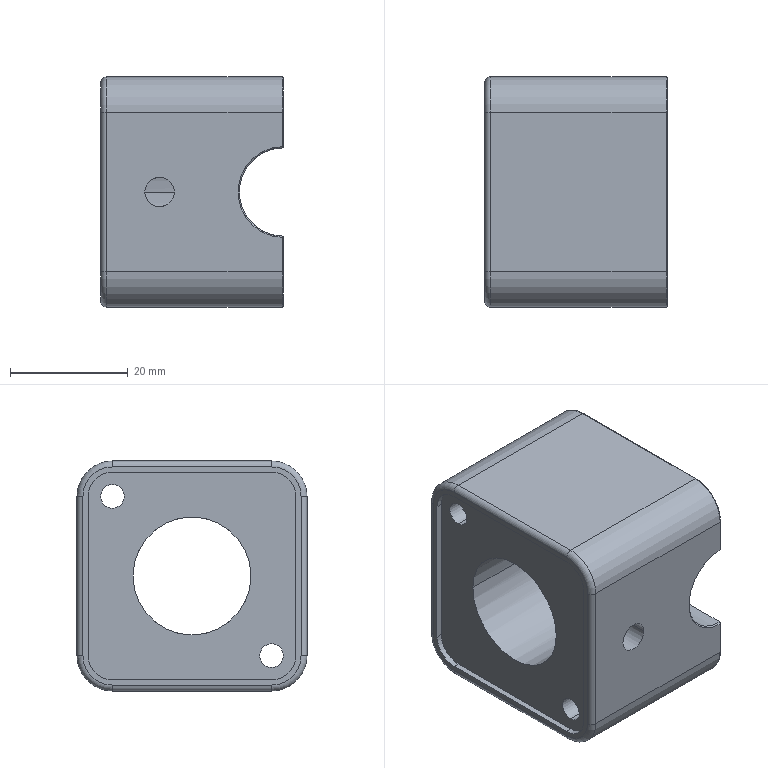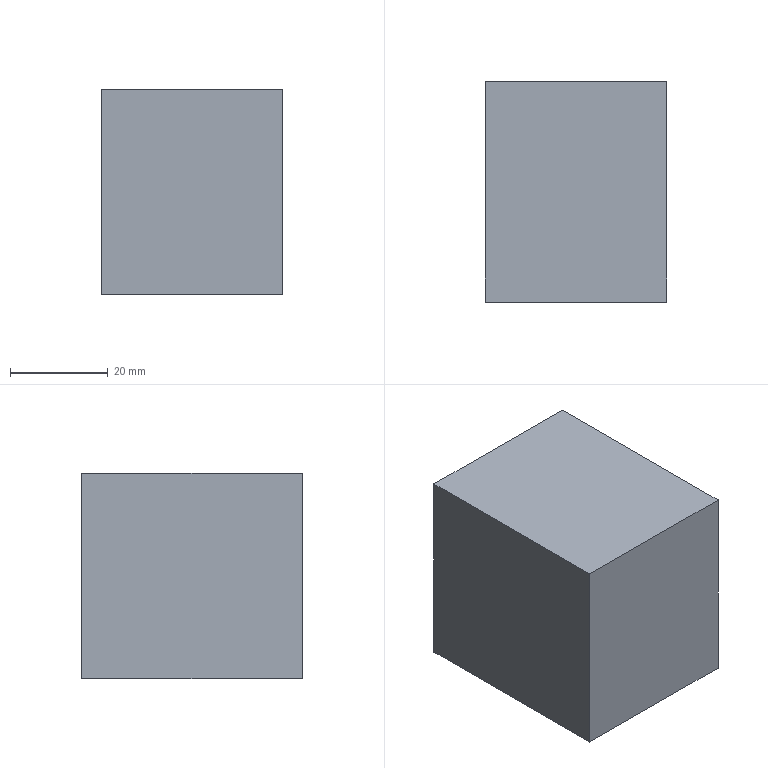CAM job | NX | 3+2 milling, drilling | part box 31 x 39 x 39 mm | stock box 37 x 45 x 42 mm
Tools:
number,name,description,diameter,corner_radius,flute_length,length,flutes
1,D50面刀,,50.0,0.0,50.0,75.0,2
2,D12C,,12.0,0.0,50.0,75.0,2
3,D10点钻,,10.0,0.0,50.0,75.0,2
4,D4.2钻头,,4.2,0.0,50.0,75.0,2
5,D3.3钻头,,3.3,0.0,50.0,75.0,2
6,M4丝锥,,4.0,0.0,50.0,75.0,2
7,D5精刀,,5.0,0.0,50.0,75.0,2
8,R0.5,,1.0,0.5,50.0,75.0,2
Operations:
program,operation,operation_type,tool,method,geometry_group,spindle_rpm,surface_speed,feed_per_tooth,feed_cut,feed_plunge,cut_length_mm,path_length_mm,cut_time_min,machine_time_min
11.NC,FACE_MILLING,FaceMilling,D50面刀,MILL_ROUGH,W1,3500.0,549.0,0.1143,800.0,60.0,141.2,161.2,0.1998,0.2018
11.NC,ADAPTIVE_MILLING,CavityMilling,D12C,MILL_ROUGH,W1,6500.0,245.0,0.1538,2000.0,60.0,604.511,682.711,0.3033,0.3111
11.NC,HOLE_MILLING,CylinderMilling,D12C,MILL_ROUGH,W1,6500.0,245.0,0.0385,500.0,60.0,800.519,851.519,1.609,1.614
11.NC,PLANAR_PROFILE,PlanarMilling,D12C,METHOD,W1,3500.0,131.0,0.1143,800.0,100.0,198.823,276.823,0.2485,0.2563
11.NC,PLANAR_PROFILE_COPY,PlanarMilling,D12C,METHOD,W1,4500.0,169.0,0.0333,300.0,100.0,32.617,112.618,0.1087,0.1167
11.NC,PLANAR_PROFILE_COPY_COPY,PlanarMilling,D10点钻,METHOD,W1,3500.0,131.0,0.1143,800.0,100.0,60.684,79.684,0.0759,0.0778
11.NC,DRILLING,Operation,D10点钻,DRILL_METHOD,W1,1200.0,37.0,0.1042,250.0,0.0,13.2,70.701,0.0528,0.0586
11.NC,DRILLING_COPY,Operation,D10点钻,DRILL_METHOD,W1,1200.0,37.0,0.1042,250.0,0.0,10.0,64.301,0.04,0.0454
11.NC,DRILLING_COPY_1,Operation,D4.2钻头,DRILL_METHOD,W1,2000.0,26.0,0.0625,250.0,0.0,72.0,188.301,0.288,0.2996
11.NC,DRILLING_COPY_COPY,Operation,D3.3钻头,DRILL_METHOD,W1,1200.0,37.0,0.1042,250.0,0.0,29.0,102.301,0.116,0.1233
11.NC,DRILLING_COPY_COPY_COPY,Operation,M4丝锥,DRILL_METHOD,W1,400.0,5.0,0.0009,0.7,0.0,26.0,96.301,37.143,37.15
11.NC,HOLE_MILLING_1,CylinderMilling,D5精刀,MILL_FINISH,W1,4500.0,70.0,0.0889,800.0,100.0,306.233,403.816,0.3828,0.3925
11.NC,ZLEVEL_PROFILE,ZLevelMilling,R0.5,MILL_FINISH,W1,4500.0,14.0,0.1667,1500.0,100.0,1178.274,1249.107,0.7855,0.7926
G55,FACE_MILLING_COPY,FaceMilling,D50面刀,MILL_ROUGH,W2,3500.0,549.0,0.1143,800.0,60.0,141.2,157.1,0.1998,0.2014
G55,FACE_MILLING_COPY_COPY,FaceMilling,D50面刀,MILL_ROUGH,W2,3500.0,549.0,0.1143,800.0,60.0,141.2,157.2,0.1998,0.2014
G55,PLANAR_MILL,PlanarMilling,D5精刀,MILL_ROUGH,W2,4500.0,169.0,0.1111,1000.0,60.0,436.625,454.625,0.438,0.4398
G55,PLANAR_MILL_COPY,PlanarMilling,D5精刀,MILL_FINISH,W2,4500.0,169.0,0.0667,600.0,100.0,358.453,376.453,0.5974,0.5992
G55,PLANAR_PROFILE_1,PlanarMilling,R0.5,MILL_FINISH,W2,4500.0,14.0,0.0889,800.0,100.0,143.767,158.367,0.1797,0.1812
G55,ZLEVEL_PROFILE_COPY,ZLevelMilling,R0.5,MILL_FINISH,W2,4500.0,14.0,0.1667,1500.0,100.0,7308.078,7323.098,4.872,4.874
G56,DRILLING_1,Operation,D10点钻,DRILL_METHOD,MCS_3,1200.0,37.0,0.1042,250.0,0.0,5.5,14.0,0.022,0.0228
G56,DRILLING_1_COPY,Operation,D4.2钻头,DRILL_METHOD,MCS_3,1200.0,37.0,0.1042,250.0,0.0,16.0,35.0,0.064,0.0659
G56,DRILLING_1_COPY_COPY,Operation,D5精刀,DRILL_METHOD,MCS_3,1600.0,25.0,0.0625,200.0,0.0,14.0,31.0,0.07,0.0717
G56,HOLE_MILLING_2,CylinderMilling,D12C,MILL_FINISH,MCS_3,4500.0,169.0,0.0444,400.0,100.0,732.663,791.663,1.832,1.838
G56,HOLE_MILLING_2_COPY,CylinderMilling,D12C,MILL_FINISH,MCS_3,4500.0,169.0,0.0222,200.0,100.0,14.137,112.537,0.0707,0.0805